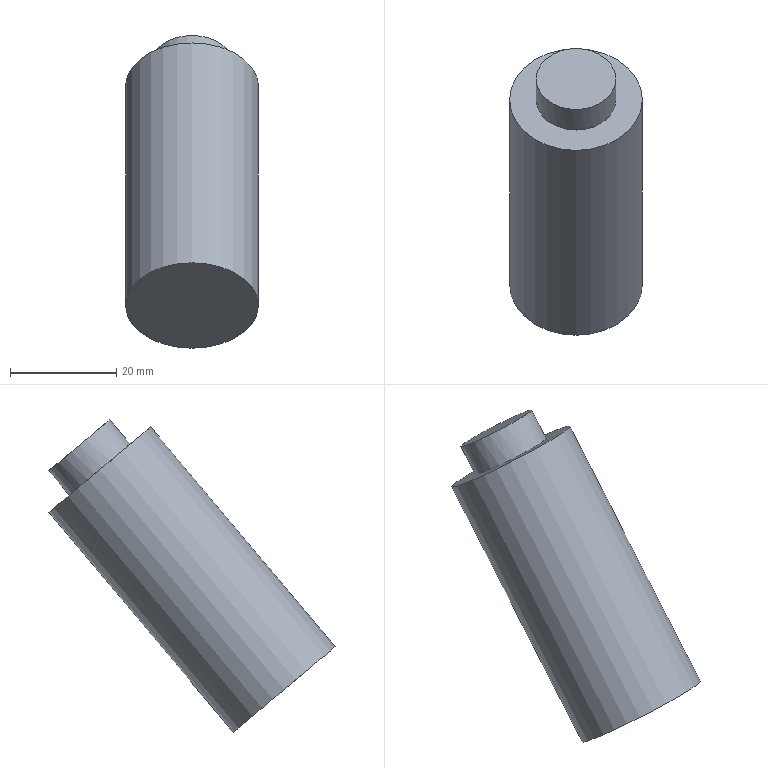Part | NX | features solid 2 | 1 solid | 5 faces | box 25 x 53.888 x 58.818 mm | volume 27567 mm3 | plane 3 | cylinder 2 | commonest cylinder face diameters 15 x1 25 x1
STEP:
#1=CARTESIAN_POINT('',(305.,400.891,-55.072));
#2=VERTEX_POINT('',#1);
#3=CARTESIAN_POINT('',(305.,410.467,-63.107));
#4=DIRECTION('',(0.,0.6428,0.766));
#5=DIRECTION('',(0.,-0.766,0.6428));
#6=AXIS2_PLACEMENT_3D('',#3,#4,#5);
#7=CIRCLE('',#6,12.5);
#8=EDGE_CURVE('',#2,#2,#7,.T.);
#9=ORIENTED_EDGE('',*,*,#8,.T.);
#10=EDGE_LOOP('',(#9));
#11=FACE_BOUND('',#10,.T.);
#12=CARTESIAN_POINT('',(305.,404.721,-58.286));
#13=VERTEX_POINT('',#12);
#14=CARTESIAN_POINT('',(305.,410.467,-63.107));
#15=DIRECTION('',(0.,0.6428,0.766));
#16=DIRECTION('',(0.,-0.766,0.6428));
#17=AXIS2_PLACEMENT_3D('',#14,#15,#16);
#18=CIRCLE('',#17,7.5);
#19=EDGE_CURVE('',#13,#13,#18,.T.);
#20=ORIENTED_EDGE('',*,*,#19,.F.);
#21=EDGE_LOOP('',(#20));
#22=FACE_BOUND('',#21,.T.);
#23=CARTESIAN_POINT('',(305.,410.467,-63.107));
#24=DIRECTION('',(0.,0.6428,0.766));
#25=DIRECTION('',(0.,-0.766,0.6428));
#26=AXIS2_PLACEMENT_3D('',#23,#24,#25);
#27=PLANE('',#26);
#28=ADVANCED_FACE('',(#11,#22),#27,.T.);
#29=ORIENTED_EDGE('',*,*,#8,.F.);
#30=EDGE_LOOP('',(#29));
#31=FACE_BOUND('',#30,.T.);
#32=CARTESIAN_POINT('',(292.5,375.756,-104.473));
#33=VERTEX_POINT('',#32);
#34=CARTESIAN_POINT('',(305.,375.756,-104.473));
#35=DIRECTION('',(0.,0.6428,0.766));
#36=DIRECTION('',(-1.,0.,0.));
#37=AXIS2_PLACEMENT_3D('',#34,#35,#36);
#38=CIRCLE('',#37,12.5);
#39=EDGE_CURVE('',#33,#33,#38,.T.);
#40=ORIENTED_EDGE('',*,*,#39,.T.);
#41=EDGE_LOOP('',(#40));
#42=FACE_BOUND('',#41,.T.);
#43=CARTESIAN_POINT('',(305.,411.109,-62.341));
#44=DIRECTION('',(0.,-0.6428,-0.766));
#45=DIRECTION('',(0.,0.766,-0.6428));
#46=AXIS2_PLACEMENT_3D('',#43,#44,#45);
#47=CYLINDRICAL_SURFACE('',#46,12.5);
#48=ADVANCED_FACE('',(#31,#42),#47,.T.);
#49=ORIENTED_EDGE('',*,*,#39,.F.);
#50=EDGE_LOOP('',(#49));
#51=FACE_BOUND('',#50,.T.);
#52=CARTESIAN_POINT('',(305.,375.756,-104.473));
#53=DIRECTION('',(0.,0.6428,0.766));
#54=DIRECTION('',(0.,-0.766,0.6428));
#55=AXIS2_PLACEMENT_3D('',#52,#53,#54);
#56=PLANE('',#55);
#57=ADVANCED_FACE('',(#51),#56,.F.);
#58=CARTESIAN_POINT('',(312.5,414.323,-58.511));
#59=VERTEX_POINT('',#58);
#60=CARTESIAN_POINT('',(305.,414.323,-58.511));
#61=DIRECTION('',(0.,-0.6428,-0.766));
#62=DIRECTION('',(1.,0.,0.));
#63=AXIS2_PLACEMENT_3D('',#60,#61,#62);
#64=CIRCLE('',#63,7.5);
#65=EDGE_CURVE('',#59,#59,#64,.F.);
#66=ORIENTED_EDGE('',*,*,#65,.F.);
#67=EDGE_LOOP('',(#66));
#68=FACE_BOUND('',#67,.T.);
#69=ORIENTED_EDGE('',*,*,#19,.T.);
#70=EDGE_LOOP('',(#69));
#71=FACE_BOUND('',#70,.T.);
#72=CARTESIAN_POINT('',(305.,416.894,-55.447));
#73=DIRECTION('',(0.,-0.6428,-0.766));
#74=DIRECTION('',(0.,0.766,-0.6428));
#75=AXIS2_PLACEMENT_3D('',#72,#73,#74);
#76=CYLINDRICAL_SURFACE('',#75,7.5);
#77=ADVANCED_FACE('',(#68,#71),#76,.T.);
#78=ORIENTED_EDGE('',*,*,#65,.T.);
#79=EDGE_LOOP('',(#78));
#80=FACE_BOUND('',#79,.T.);
#81=CARTESIAN_POINT('',(305.,414.323,-58.511));
#82=DIRECTION('',(0.,0.6428,0.766));
#83=DIRECTION('',(0.,-0.766,0.6428));
#84=AXIS2_PLACEMENT_3D('',#81,#82,#83);
#85=PLANE('',#84);
#86=ADVANCED_FACE('',(#80),#85,.T.);
#87=CLOSED_SHELL('',(#28,#48,#57,#77,#86));
#88=MANIFOLD_SOLID_BREP('',#87);
#89=(LENGTH_UNIT()NAMED_UNIT(*)SI_UNIT(.MILLI.,.METRE.));
#90=UNCERTAINTY_MEASURE_WITH_UNIT(LENGTH_MEASURE(0.00001),#89,'','');
#91=(NAMED_UNIT(*)PLANE_ANGLE_UNIT()SI_UNIT($,.RADIAN.));
#92=(NAMED_UNIT(*)SI_UNIT($,.STERADIAN.)SOLID_ANGLE_UNIT());
#93=(GEOMETRIC_REPRESENTATION_CONTEXT(3)GLOBAL_UNCERTAINTY_ASSIGNED_CONTEXT((#90))GLOBAL_UNIT_ASSIGNED_CONTEXT((#89,#91,#92))REPRESENTATION_CONTEXT('',''));
#94=ADVANCED_BREP_SHAPE_REPRESENTATION('',(#88),#93);